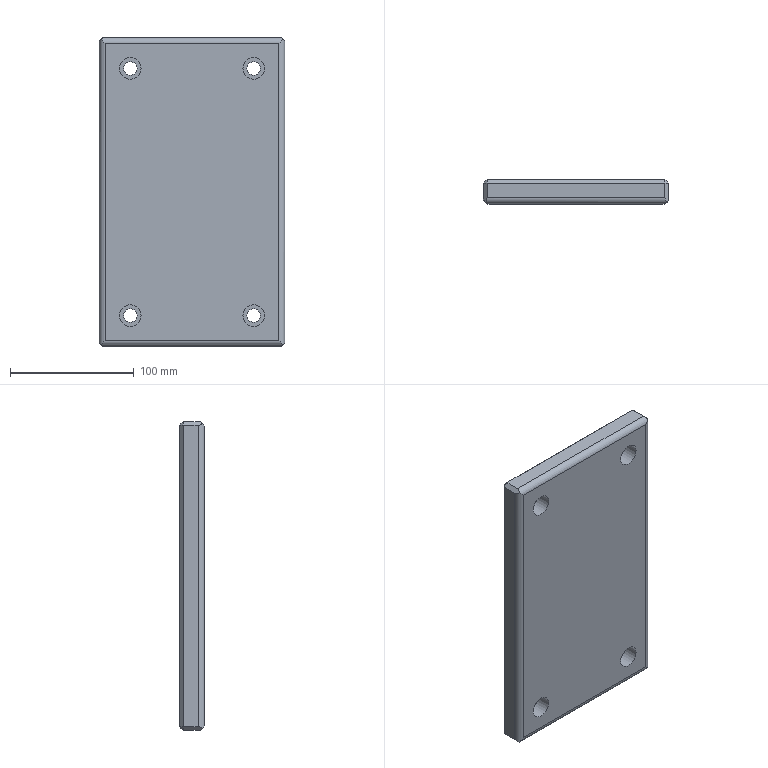Part | NX | features MAIN_BODY 2 | 1 solid | 34 faces | box 150 x 20 x 250 mm | volume 727336 mm3 | plane 22 | cylinder 12 | commonest cylinder face diameters 10 x4 11 x4 17.5 x4
STEP:
#1=CARTESIAN_POINT('',(1390.5,-413.,-220.));
#2=VERTEX_POINT('',#1);
#3=CARTESIAN_POINT('',(1390.5,-425.,-220.));
#4=VERTEX_POINT('',#3);
#5=CARTESIAN_POINT('',(1390.5,-410.,-220.));
#6=DIRECTION('',(0.,-1.,0.));
#7=VECTOR('',#6,1000.);
#8=LINE('',#5,#7);
#9=EDGE_CURVE('',#2,#4,#8,.T.);
#10=ORIENTED_EDGE('',*,*,#9,.F.);
#11=CARTESIAN_POINT('',(1534.5,-413.,-220.));
#12=VERTEX_POINT('',#11);
#13=CARTESIAN_POINT('',(1387.5,-413.,-220.));
#14=DIRECTION('',(-1.,0.,0.));
#15=VECTOR('',#14,1000.);
#16=LINE('',#13,#15);
#17=EDGE_CURVE('',#12,#2,#16,.T.);
#18=ORIENTED_EDGE('',*,*,#17,.F.);
#19=CARTESIAN_POINT('',(1534.5,-425.,-220.));
#20=VERTEX_POINT('',#19);
#21=CARTESIAN_POINT('',(1534.5,-410.,-220.));
#22=DIRECTION('',(0.,1.,0.));
#23=VECTOR('',#22,1000.);
#24=LINE('',#21,#23);
#25=EDGE_CURVE('',#20,#12,#24,.T.);
#26=ORIENTED_EDGE('',*,*,#25,.F.);
#27=CARTESIAN_POINT('',(1534.5,-425.,-220.));
#28=DIRECTION('',(1.,0.,0.));
#29=VECTOR('',#28,1000.);
#30=LINE('',#27,#29);
#31=EDGE_CURVE('',#4,#20,#30,.T.);
#32=ORIENTED_EDGE('',*,*,#31,.F.);
#33=EDGE_LOOP('',(#10,#18,#26,#32));
#34=FACE_BOUND('',#33,.T.);
#35=CARTESIAN_POINT('',(1387.5,-410.,-220.));
#36=DIRECTION('',(0.,0.,1.));
#37=DIRECTION('',(0.,1.,0.));
#38=AXIS2_PLACEMENT_3D('',#35,#36,#37);
#39=PLANE('',#38);
#40=ADVANCED_FACE('',(#34),#39,.F.);
#41=CARTESIAN_POINT('',(1537.5,-413.,-217.));
#42=VERTEX_POINT('',#41);
#43=CARTESIAN_POINT('',(1537.5,-425.,-217.));
#44=VERTEX_POINT('',#43);
#45=CARTESIAN_POINT('',(1537.5,-410.,-217.));
#46=DIRECTION('',(0.,-1.,0.));
#47=VECTOR('',#46,1000.);
#48=LINE('',#45,#47);
#49=EDGE_CURVE('',#42,#44,#48,.T.);
#50=ORIENTED_EDGE('',*,*,#49,.F.);
#51=CARTESIAN_POINT('',(1537.5,-413.,27.));
#52=VERTEX_POINT('',#51);
#53=CARTESIAN_POINT('',(1537.5,-413.,-220.));
#54=DIRECTION('',(0.,0.,-1.));
#55=VECTOR('',#54,1000.);
#56=LINE('',#53,#55);
#57=EDGE_CURVE('',#52,#42,#56,.T.);
#58=ORIENTED_EDGE('',*,*,#57,.F.);
#59=CARTESIAN_POINT('',(1537.5,-425.,27.));
#60=VERTEX_POINT('',#59);
#61=CARTESIAN_POINT('',(1537.5,-410.,27.));
#62=DIRECTION('',(0.,1.,0.));
#63=VECTOR('',#62,1000.);
#64=LINE('',#61,#63);
#65=EDGE_CURVE('',#60,#52,#64,.T.);
#66=ORIENTED_EDGE('',*,*,#65,.F.);
#67=CARTESIAN_POINT('',(1537.5,-425.,27.));
#68=DIRECTION('',(0.,0.,1.));
#69=VECTOR('',#68,1000.);
#70=LINE('',#67,#69);
#71=EDGE_CURVE('',#44,#60,#70,.T.);
#72=ORIENTED_EDGE('',*,*,#71,.F.);
#73=EDGE_LOOP('',(#50,#58,#66,#72));
#74=FACE_BOUND('',#73,.T.);
#75=CARTESIAN_POINT('',(1537.5,-410.,-220.));
#76=DIRECTION('',(-1.,0.,0.));
#77=DIRECTION('',(0.,0.,1.));
#78=AXIS2_PLACEMENT_3D('',#75,#76,#77);
#79=PLANE('',#78);
#80=ADVANCED_FACE('',(#74),#79,.F.);
#81=CARTESIAN_POINT('',(1534.5,-413.,30.));
#82=VERTEX_POINT('',#81);
#83=CARTESIAN_POINT('',(1534.5,-425.,30.));
#84=VERTEX_POINT('',#83);
#85=CARTESIAN_POINT('',(1534.5,-410.,30.));
#86=DIRECTION('',(0.,-1.,0.));
#87=VECTOR('',#86,1000.);
#88=LINE('',#85,#87);
#89=EDGE_CURVE('',#82,#84,#88,.T.);
#90=ORIENTED_EDGE('',*,*,#89,.F.);
#91=CARTESIAN_POINT('',(1390.5,-413.,30.));
#92=VERTEX_POINT('',#91);
#93=CARTESIAN_POINT('',(1537.5,-413.,30.));
#94=DIRECTION('',(1.,0.,0.));
#95=VECTOR('',#94,1000.);
#96=LINE('',#93,#95);
#97=EDGE_CURVE('',#92,#82,#96,.T.);
#98=ORIENTED_EDGE('',*,*,#97,.F.);
#99=CARTESIAN_POINT('',(1390.5,-425.,30.));
#100=VERTEX_POINT('',#99);
#101=CARTESIAN_POINT('',(1390.5,-410.,30.));
#102=DIRECTION('',(0.,1.,0.));
#103=VECTOR('',#102,1000.);
#104=LINE('',#101,#103);
#105=EDGE_CURVE('',#100,#92,#104,.T.);
#106=ORIENTED_EDGE('',*,*,#105,.F.);
#107=CARTESIAN_POINT('',(1390.5,-425.,30.));
#108=DIRECTION('',(-1.,0.,0.));
#109=VECTOR('',#108,1000.);
#110=LINE('',#107,#109);
#111=EDGE_CURVE('',#84,#100,#110,.T.);
#112=ORIENTED_EDGE('',*,*,#111,.F.);
#113=EDGE_LOOP('',(#90,#98,#106,#112));
#114=FACE_BOUND('',#113,.T.);
#115=CARTESIAN_POINT('',(1537.5,-410.,30.));
#116=DIRECTION('',(0.,0.,-1.));
#117=DIRECTION('',(-1.,0.,0.));
#118=AXIS2_PLACEMENT_3D('',#115,#116,#117);
#119=PLANE('',#118);
#120=ADVANCED_FACE('',(#114),#119,.F.);
#121=CARTESIAN_POINT('',(1387.5,-413.,27.));
#122=VERTEX_POINT('',#121);
#123=CARTESIAN_POINT('',(1387.5,-425.,27.));
#124=VERTEX_POINT('',#123);
#125=CARTESIAN_POINT('',(1387.5,-410.,27.));
#126=DIRECTION('',(0.,-1.,0.));
#127=VECTOR('',#126,1000.);
#128=LINE('',#125,#127);
#129=EDGE_CURVE('',#122,#124,#128,.T.);
#130=ORIENTED_EDGE('',*,*,#129,.F.);
#131=CARTESIAN_POINT('',(1387.5,-413.,-217.));
#132=VERTEX_POINT('',#131);
#133=CARTESIAN_POINT('',(1387.5,-413.,30.));
#134=DIRECTION('',(0.,0.,1.));
#135=VECTOR('',#134,1000.);
#136=LINE('',#133,#135);
#137=EDGE_CURVE('',#132,#122,#136,.T.);
#138=ORIENTED_EDGE('',*,*,#137,.F.);
#139=CARTESIAN_POINT('',(1387.5,-425.,-217.));
#140=VERTEX_POINT('',#139);
#141=CARTESIAN_POINT('',(1387.5,-410.,-217.));
#142=DIRECTION('',(0.,1.,0.));
#143=VECTOR('',#142,1000.);
#144=LINE('',#141,#143);
#145=EDGE_CURVE('',#140,#132,#144,.T.);
#146=ORIENTED_EDGE('',*,*,#145,.F.);
#147=CARTESIAN_POINT('',(1387.5,-425.,-217.));
#148=DIRECTION('',(0.,0.,-1.));
#149=VECTOR('',#148,1000.);
#150=LINE('',#147,#149);
#151=EDGE_CURVE('',#124,#140,#150,.T.);
#152=ORIENTED_EDGE('',*,*,#151,.F.);
#153=EDGE_LOOP('',(#130,#138,#146,#152));
#154=FACE_BOUND('',#153,.T.);
#155=CARTESIAN_POINT('',(1387.5,-410.,30.));
#156=DIRECTION('',(1.,0.,0.));
#157=DIRECTION('',(0.,0.,-1.));
#158=AXIS2_PLACEMENT_3D('',#155,#156,#157);
#159=PLANE('',#158);
#160=ADVANCED_FACE('',(#154),#159,.F.);
#161=CARTESIAN_POINT('',(1390.5,-410.,27.));
#162=VERTEX_POINT('',#161);
#163=CARTESIAN_POINT('',(1390.5,-410.,-217.));
#164=VERTEX_POINT('',#163);
#165=CARTESIAN_POINT('',(1390.5,-410.,-220.));
#166=DIRECTION('',(0.,0.,-1.));
#167=VECTOR('',#166,1000.);
#168=LINE('',#165,#167);
#169=EDGE_CURVE('',#162,#164,#168,.T.);
#170=ORIENTED_EDGE('',*,*,#169,.F.);
#171=CARTESIAN_POINT('',(1534.5,-410.,27.));
#172=VERTEX_POINT('',#171);
#173=CARTESIAN_POINT('',(1387.5,-410.,27.));
#174=DIRECTION('',(-1.,0.,0.));
#175=VECTOR('',#174,1000.);
#176=LINE('',#173,#175);
#177=EDGE_CURVE('',#172,#162,#176,.T.);
#178=ORIENTED_EDGE('',*,*,#177,.F.);
#179=CARTESIAN_POINT('',(1534.5,-410.,-217.));
#180=VERTEX_POINT('',#179);
#181=CARTESIAN_POINT('',(1534.5,-410.,-220.));
#182=DIRECTION('',(0.,0.,1.));
#183=VECTOR('',#182,1000.);
#184=LINE('',#181,#183);
#185=EDGE_CURVE('',#180,#172,#184,.T.);
#186=ORIENTED_EDGE('',*,*,#185,.F.);
#187=CARTESIAN_POINT('',(1387.5,-410.,-217.));
#188=DIRECTION('',(1.,0.,0.));
#189=VECTOR('',#188,1000.);
#190=LINE('',#187,#189);
#191=EDGE_CURVE('',#164,#180,#190,.T.);
#192=ORIENTED_EDGE('',*,*,#191,.F.);
#193=EDGE_LOOP('',(#170,#178,#186,#192));
#194=FACE_BOUND('',#193,.T.);
#195=CARTESIAN_POINT('',(1518.,-410.,-195.));
#196=VERTEX_POINT('',#195);
#197=CARTESIAN_POINT('',(1512.5,-410.,-195.));
#198=DIRECTION('',(0.,1.,0.));
#199=DIRECTION('',(1.,0.,0.));
#200=AXIS2_PLACEMENT_3D('',#197,#198,#199);
#201=CIRCLE('',#200,5.5);
#202=EDGE_CURVE('',#196,#196,#201,.T.);
#203=ORIENTED_EDGE('',*,*,#202,.F.);
#204=EDGE_LOOP('',(#203));
#205=FACE_BOUND('',#204,.T.);
#206=CARTESIAN_POINT('',(1418.,-410.,-195.));
#207=VERTEX_POINT('',#206);
#208=CARTESIAN_POINT('',(1412.5,-410.,-195.));
#209=DIRECTION('',(0.,1.,0.));
#210=DIRECTION('',(1.,0.,0.));
#211=AXIS2_PLACEMENT_3D('',#208,#209,#210);
#212=CIRCLE('',#211,5.5);
#213=EDGE_CURVE('',#207,#207,#212,.T.);
#214=ORIENTED_EDGE('',*,*,#213,.F.);
#215=EDGE_LOOP('',(#214));
#216=FACE_BOUND('',#215,.T.);
#217=CARTESIAN_POINT('',(1418.,-410.,5.));
#218=VERTEX_POINT('',#217);
#219=CARTESIAN_POINT('',(1412.5,-410.,5.));
#220=DIRECTION('',(0.,1.,0.));
#221=DIRECTION('',(1.,0.,0.));
#222=AXIS2_PLACEMENT_3D('',#219,#220,#221);
#223=CIRCLE('',#222,5.5);
#224=EDGE_CURVE('',#218,#218,#223,.T.);
#225=ORIENTED_EDGE('',*,*,#224,.F.);
#226=EDGE_LOOP('',(#225));
#227=FACE_BOUND('',#226,.T.);
#228=CARTESIAN_POINT('',(1518.,-410.,5.));
#229=VERTEX_POINT('',#228);
#230=CARTESIAN_POINT('',(1512.5,-410.,5.));
#231=DIRECTION('',(0.,1.,0.));
#232=DIRECTION('',(1.,0.,0.));
#233=AXIS2_PLACEMENT_3D('',#230,#231,#232);
#234=CIRCLE('',#233,5.5);
#235=EDGE_CURVE('',#229,#229,#234,.T.);
#236=ORIENTED_EDGE('',*,*,#235,.F.);
#237=EDGE_LOOP('',(#236));
#238=FACE_BOUND('',#237,.T.);
#239=CARTESIAN_POINT('',(1387.5,-410.,-220.));
#240=DIRECTION('',(0.,-1.,0.));
#241=DIRECTION('',(1.,0.,0.));
#242=AXIS2_PLACEMENT_3D('',#239,#240,#241);
#243=PLANE('',#242);
#244=ADVANCED_FACE('',(#194,#205,#216,#227,#238),#243,.F.);
#245=CARTESIAN_POINT('',(1392.5,-430.,25.));
#246=VERTEX_POINT('',#245);
#247=CARTESIAN_POINT('',(1532.5,-430.,25.));
#248=VERTEX_POINT('',#247);
#249=CARTESIAN_POINT('',(1534.5,-430.,25.));
#250=DIRECTION('',(-1.,0.,0.));
#251=VECTOR('',#250,1000.);
#252=LINE('',#249,#251);
#253=EDGE_CURVE('',#246,#248,#252,.F.);
#254=ORIENTED_EDGE('',*,*,#253,.F.);
#255=CARTESIAN_POINT('',(1392.5,-430.,-215.));
#256=VERTEX_POINT('',#255);
#257=CARTESIAN_POINT('',(1392.5,-430.,27.));
#258=DIRECTION('',(0.,0.,-1.));
#259=VECTOR('',#258,1000.);
#260=LINE('',#257,#259);
#261=EDGE_CURVE('',#256,#246,#260,.F.);
#262=ORIENTED_EDGE('',*,*,#261,.F.);
#263=CARTESIAN_POINT('',(1532.5,-430.,-215.));
#264=VERTEX_POINT('',#263);
#265=CARTESIAN_POINT('',(1390.5,-430.,-215.));
#266=DIRECTION('',(1.,0.,0.));
#267=VECTOR('',#266,1000.);
#268=LINE('',#265,#267);
#269=EDGE_CURVE('',#264,#256,#268,.F.);
#270=ORIENTED_EDGE('',*,*,#269,.F.);
#271=CARTESIAN_POINT('',(1532.5,-430.,-217.));
#272=DIRECTION('',(0.,0.,1.));
#273=VECTOR('',#272,1000.);
#274=LINE('',#271,#273);
#275=EDGE_CURVE('',#248,#264,#274,.F.);
#276=ORIENTED_EDGE('',*,*,#275,.F.);
#277=EDGE_LOOP('',(#254,#262,#270,#276));
#278=FACE_BOUND('',#277,.T.);
#279=CARTESIAN_POINT('',(1503.75,-430.,-195.));
#280=VERTEX_POINT('',#279);
#281=CARTESIAN_POINT('',(1512.5,-430.,-195.));
#282=DIRECTION('',(0.,-1.,0.));
#283=DIRECTION('',(-1.,0.,0.));
#284=AXIS2_PLACEMENT_3D('',#281,#282,#283);
#285=CIRCLE('',#284,8.75);
#286=EDGE_CURVE('',#280,#280,#285,.T.);
#287=ORIENTED_EDGE('',*,*,#286,.F.);
#288=EDGE_LOOP('',(#287));
#289=FACE_BOUND('',#288,.T.);
#290=CARTESIAN_POINT('',(1403.75,-430.,-195.));
#291=VERTEX_POINT('',#290);
#292=CARTESIAN_POINT('',(1412.5,-430.,-195.));
#293=DIRECTION('',(0.,-1.,0.));
#294=DIRECTION('',(-1.,0.,0.));
#295=AXIS2_PLACEMENT_3D('',#292,#293,#294);
#296=CIRCLE('',#295,8.75);
#297=EDGE_CURVE('',#291,#291,#296,.T.);
#298=ORIENTED_EDGE('',*,*,#297,.F.);
#299=EDGE_LOOP('',(#298));
#300=FACE_BOUND('',#299,.T.);
#301=CARTESIAN_POINT('',(1403.75,-430.,5.));
#302=VERTEX_POINT('',#301);
#303=CARTESIAN_POINT('',(1412.5,-430.,5.));
#304=DIRECTION('',(0.,-1.,0.));
#305=DIRECTION('',(-1.,0.,0.));
#306=AXIS2_PLACEMENT_3D('',#303,#304,#305);
#307=CIRCLE('',#306,8.75);
#308=EDGE_CURVE('',#302,#302,#307,.T.);
#309=ORIENTED_EDGE('',*,*,#308,.F.);
#310=EDGE_LOOP('',(#309));
#311=FACE_BOUND('',#310,.T.);
#312=CARTESIAN_POINT('',(1503.75,-430.,5.));
#313=VERTEX_POINT('',#312);
#314=CARTESIAN_POINT('',(1512.5,-430.,5.));
#315=DIRECTION('',(0.,-1.,0.));
#316=DIRECTION('',(-1.,0.,0.));
#317=AXIS2_PLACEMENT_3D('',#314,#315,#316);
#318=CIRCLE('',#317,8.75);
#319=EDGE_CURVE('',#313,#313,#318,.T.);
#320=ORIENTED_EDGE('',*,*,#319,.F.);
#321=EDGE_LOOP('',(#320));
#322=FACE_BOUND('',#321,.T.);
#323=CARTESIAN_POINT('',(1387.5,-430.,-220.));
#324=DIRECTION('',(0.,-1.,0.));
#325=DIRECTION('',(1.,0.,0.));
#326=AXIS2_PLACEMENT_3D('',#323,#324,#325);
#327=PLANE('',#326);
#328=ADVANCED_FACE('',(#278,#289,#300,#311,#322),#327,.T.);
#329=CARTESIAN_POINT('',(1507.,-418.,5.));
#330=VERTEX_POINT('',#329);
#331=CARTESIAN_POINT('',(1512.5,-418.,5.));
#332=DIRECTION('',(0.,-1.,0.));
#333=DIRECTION('',(-1.,0.,0.));
#334=AXIS2_PLACEMENT_3D('',#331,#332,#333);
#335=CIRCLE('',#334,5.5);
#336=EDGE_CURVE('',#330,#330,#335,.T.);
#337=ORIENTED_EDGE('',*,*,#336,.T.);
#338=EDGE_LOOP('',(#337));
#339=FACE_BOUND('',#338,.T.);
#340=ORIENTED_EDGE('',*,*,#235,.T.);
#341=EDGE_LOOP('',(#340));
#342=FACE_BOUND('',#341,.T.);
#343=CARTESIAN_POINT('',(1512.5,-380.,5.));
#344=DIRECTION('',(0.,1.,0.));
#345=DIRECTION('',(-1.,0.,0.));
#346=AXIS2_PLACEMENT_3D('',#343,#344,#345);
#347=CYLINDRICAL_SURFACE('',#346,5.5);
#348=ADVANCED_FACE('',(#339,#342),#347,.F.);
#349=ORIENTED_EDGE('',*,*,#336,.F.);
#350=EDGE_LOOP('',(#349));
#351=FACE_BOUND('',#350,.T.);
#352=CARTESIAN_POINT('',(1503.75,-418.,5.));
#353=VERTEX_POINT('',#352);
#354=CARTESIAN_POINT('',(1512.5,-418.,5.));
#355=DIRECTION('',(0.,-1.,0.));
#356=DIRECTION('',(-1.,0.,0.));
#357=AXIS2_PLACEMENT_3D('',#354,#355,#356);
#358=CIRCLE('',#357,8.75);
#359=EDGE_CURVE('',#353,#353,#358,.T.);
#360=ORIENTED_EDGE('',*,*,#359,.T.);
#361=EDGE_LOOP('',(#360));
#362=FACE_BOUND('',#361,.T.);
#363=CARTESIAN_POINT('',(1512.5,-418.,5.));
#364=DIRECTION('',(0.,1.,0.));
#365=DIRECTION('',(-1.,0.,0.));
#366=AXIS2_PLACEMENT_3D('',#363,#364,#365);
#367=PLANE('',#366);
#368=ADVANCED_FACE('',(#351,#362),#367,.F.);
#369=ORIENTED_EDGE('',*,*,#359,.F.);
#370=EDGE_LOOP('',(#369));
#371=FACE_BOUND('',#370,.T.);
#372=ORIENTED_EDGE('',*,*,#319,.T.);
#373=EDGE_LOOP('',(#372));
#374=FACE_BOUND('',#373,.T.);
#375=CARTESIAN_POINT('',(1512.5,-430.,5.));
#376=DIRECTION('',(0.,1.,0.));
#377=DIRECTION('',(-1.,0.,0.));
#378=AXIS2_PLACEMENT_3D('',#375,#376,#377);
#379=CYLINDRICAL_SURFACE('',#378,8.75);
#380=ADVANCED_FACE('',(#371,#374),#379,.F.);
#381=CARTESIAN_POINT('',(1407.,-418.,5.));
#382=VERTEX_POINT('',#381);
#383=CARTESIAN_POINT('',(1412.5,-418.,5.));
#384=DIRECTION('',(0.,-1.,0.));
#385=DIRECTION('',(-1.,0.,0.));
#386=AXIS2_PLACEMENT_3D('',#383,#384,#385);
#387=CIRCLE('',#386,5.5);
#388=EDGE_CURVE('',#382,#382,#387,.T.);
#389=ORIENTED_EDGE('',*,*,#388,.T.);
#390=EDGE_LOOP('',(#389));
#391=FACE_BOUND('',#390,.T.);
#392=ORIENTED_EDGE('',*,*,#224,.T.);
#393=EDGE_LOOP('',(#392));
#394=FACE_BOUND('',#393,.T.);
#395=CARTESIAN_POINT('',(1412.5,-380.,5.));
#396=DIRECTION('',(0.,1.,0.));
#397=DIRECTION('',(-1.,0.,0.));
#398=AXIS2_PLACEMENT_3D('',#395,#396,#397);
#399=CYLINDRICAL_SURFACE('',#398,5.5);
#400=ADVANCED_FACE('',(#391,#394),#399,.F.);
#401=ORIENTED_EDGE('',*,*,#388,.F.);
#402=EDGE_LOOP('',(#401));
#403=FACE_BOUND('',#402,.T.);
#404=CARTESIAN_POINT('',(1403.75,-418.,5.));
#405=VERTEX_POINT('',#404);
#406=CARTESIAN_POINT('',(1412.5,-418.,5.));
#407=DIRECTION('',(0.,-1.,0.));
#408=DIRECTION('',(-1.,0.,0.));
#409=AXIS2_PLACEMENT_3D('',#406,#407,#408);
#410=CIRCLE('',#409,8.75);
#411=EDGE_CURVE('',#405,#405,#410,.T.);
#412=ORIENTED_EDGE('',*,*,#411,.T.);
#413=EDGE_LOOP('',(#412));
#414=FACE_BOUND('',#413,.T.);
#415=CARTESIAN_POINT('',(1412.5,-418.,5.));
#416=DIRECTION('',(0.,1.,0.));
#417=DIRECTION('',(-1.,0.,0.));
#418=AXIS2_PLACEMENT_3D('',#415,#416,#417);
#419=PLANE('',#418);
#420=ADVANCED_FACE('',(#403,#414),#419,.F.);
#421=ORIENTED_EDGE('',*,*,#411,.F.);
#422=EDGE_LOOP('',(#421));
#423=FACE_BOUND('',#422,.T.);
#424=ORIENTED_EDGE('',*,*,#308,.T.);
#425=EDGE_LOOP('',(#424));
#426=FACE_BOUND('',#425,.T.);
#427=CARTESIAN_POINT('',(1412.5,-430.,5.));
#428=DIRECTION('',(0.,1.,0.));
#429=DIRECTION('',(-1.,0.,0.));
#430=AXIS2_PLACEMENT_3D('',#427,#428,#429);
#431=CYLINDRICAL_SURFACE('',#430,8.75);
#432=ADVANCED_FACE('',(#423,#426),#431,.F.);
#433=CARTESIAN_POINT('',(1407.,-418.,-195.));
#434=VERTEX_POINT('',#433);
#435=CARTESIAN_POINT('',(1412.5,-418.,-195.));
#436=DIRECTION('',(0.,-1.,0.));
#437=DIRECTION('',(-1.,0.,0.));
#438=AXIS2_PLACEMENT_3D('',#435,#436,#437);
#439=CIRCLE('',#438,5.5);
#440=EDGE_CURVE('',#434,#434,#439,.T.);
#441=ORIENTED_EDGE('',*,*,#440,.T.);
#442=EDGE_LOOP('',(#441));
#443=FACE_BOUND('',#442,.T.);
#444=ORIENTED_EDGE('',*,*,#213,.T.);
#445=EDGE_LOOP('',(#444));
#446=FACE_BOUND('',#445,.T.);
#447=CARTESIAN_POINT('',(1412.5,-380.,-195.));
#448=DIRECTION('',(0.,1.,0.));
#449=DIRECTION('',(-1.,0.,0.));
#450=AXIS2_PLACEMENT_3D('',#447,#448,#449);
#451=CYLINDRICAL_SURFACE('',#450,5.5);
#452=ADVANCED_FACE('',(#443,#446),#451,.F.);
#453=ORIENTED_EDGE('',*,*,#440,.F.);
#454=EDGE_LOOP('',(#453));
#455=FACE_BOUND('',#454,.T.);
#456=CARTESIAN_POINT('',(1403.75,-418.,-195.));
#457=VERTEX_POINT('',#456);
#458=CARTESIAN_POINT('',(1412.5,-418.,-195.));
#459=DIRECTION('',(0.,-1.,0.));
#460=DIRECTION('',(-1.,0.,0.));
#461=AXIS2_PLACEMENT_3D('',#458,#459,#460);
#462=CIRCLE('',#461,8.75);
#463=EDGE_CURVE('',#457,#457,#462,.T.);
#464=ORIENTED_EDGE('',*,*,#463,.T.);
#465=EDGE_LOOP('',(#464));
#466=FACE_BOUND('',#465,.T.);
#467=CARTESIAN_POINT('',(1412.5,-418.,-195.));
#468=DIRECTION('',(0.,1.,0.));
#469=DIRECTION('',(-1.,0.,0.));
#470=AXIS2_PLACEMENT_3D('',#467,#468,#469);
#471=PLANE('',#470);
#472=ADVANCED_FACE('',(#455,#466),#471,.F.);
#473=ORIENTED_EDGE('',*,*,#463,.F.);
#474=EDGE_LOOP('',(#473));
#475=FACE_BOUND('',#474,.T.);
#476=ORIENTED_EDGE('',*,*,#297,.T.);
#477=EDGE_LOOP('',(#476));
#478=FACE_BOUND('',#477,.T.);
#479=CARTESIAN_POINT('',(1412.5,-430.,-195.));
#480=DIRECTION('',(0.,1.,0.));
#481=DIRECTION('',(-1.,0.,0.));
#482=AXIS2_PLACEMENT_3D('',#479,#480,#481);
#483=CYLINDRICAL_SURFACE('',#482,8.75);
#484=ADVANCED_FACE('',(#475,#478),#483,.F.);
#485=CARTESIAN_POINT('',(1507.,-418.,-195.));
#486=VERTEX_POINT('',#485);
#487=CARTESIAN_POINT('',(1512.5,-418.,-195.));
#488=DIRECTION('',(0.,-1.,0.));
#489=DIRECTION('',(-1.,0.,0.));
#490=AXIS2_PLACEMENT_3D('',#487,#488,#489);
#491=CIRCLE('',#490,5.5);
#492=EDGE_CURVE('',#486,#486,#491,.T.);
#493=ORIENTED_EDGE('',*,*,#492,.T.);
#494=EDGE_LOOP('',(#493));
#495=FACE_BOUND('',#494,.T.);
#496=ORIENTED_EDGE('',*,*,#202,.T.);
#497=EDGE_LOOP('',(#496));
#498=FACE_BOUND('',#497,.T.);
#499=CARTESIAN_POINT('',(1512.5,-380.,-195.));
#500=DIRECTION('',(0.,1.,0.));
#501=DIRECTION('',(-1.,0.,0.));
#502=AXIS2_PLACEMENT_3D('',#499,#500,#501);
#503=CYLINDRICAL_SURFACE('',#502,5.5);
#504=ADVANCED_FACE('',(#495,#498),#503,.F.);
#505=ORIENTED_EDGE('',*,*,#492,.F.);
#506=EDGE_LOOP('',(#505));
#507=FACE_BOUND('',#506,.T.);
#508=CARTESIAN_POINT('',(1503.75,-418.,-195.));
#509=VERTEX_POINT('',#508);
#510=CARTESIAN_POINT('',(1512.5,-418.,-195.));
#511=DIRECTION('',(0.,-1.,0.));
#512=DIRECTION('',(-1.,0.,0.));
#513=AXIS2_PLACEMENT_3D('',#510,#511,#512);
#514=CIRCLE('',#513,8.75);
#515=EDGE_CURVE('',#509,#509,#514,.T.);
#516=ORIENTED_EDGE('',*,*,#515,.T.);
#517=EDGE_LOOP('',(#516));
#518=FACE_BOUND('',#517,.T.);
#519=CARTESIAN_POINT('',(1512.5,-418.,-195.));
#520=DIRECTION('',(0.,1.,0.));
#521=DIRECTION('',(-1.,0.,0.));
#522=AXIS2_PLACEMENT_3D('',#519,#520,#521);
#523=PLANE('',#522);
#524=ADVANCED_FACE('',(#507,#518),#523,.F.);
#525=ORIENTED_EDGE('',*,*,#515,.F.);
#526=EDGE_LOOP('',(#525));
#527=FACE_BOUND('',#526,.T.);
#528=ORIENTED_EDGE('',*,*,#286,.T.);
#529=EDGE_LOOP('',(#528));
#530=FACE_BOUND('',#529,.T.);
#531=CARTESIAN_POINT('',(1512.5,-430.,-195.));
#532=DIRECTION('',(0.,1.,0.));
#533=DIRECTION('',(-1.,0.,0.));
#534=AXIS2_PLACEMENT_3D('',#531,#532,#533);
#535=CYLINDRICAL_SURFACE('',#534,8.75);
#536=ADVANCED_FACE('',(#527,#530),#535,.F.);
#537=CARTESIAN_POINT('',(1389.,-428.571,28.5));
#538=VERTEX_POINT('',#537);
#539=CARTESIAN_POINT('',(1385.5,-425.,25.));
#540=DIRECTION('',(-0.7071,0.,0.7071));
#541=DIRECTION('',(0.7071,0.,0.7071));
#542=AXIS2_PLACEMENT_3D('',#539,#540,#541);
#543=ELLIPSE('',#542,7.071,5.);
#544=EDGE_CURVE('',#100,#538,#543,.F.);
#545=ORIENTED_EDGE('',*,*,#544,.F.);
#546=ORIENTED_EDGE('',*,*,#105,.T.);
#547=CARTESIAN_POINT('',(1387.5,-413.,27.));
#548=DIRECTION('',(0.7071,0.,0.7071));
#549=VECTOR('',#548,1000.);
#550=LINE('',#547,#549);
#551=EDGE_CURVE('',#92,#122,#550,.F.);
#552=ORIENTED_EDGE('',*,*,#551,.T.);
#553=ORIENTED_EDGE('',*,*,#129,.T.);
#554=CARTESIAN_POINT('',(1392.5,-425.,32.));
#555=DIRECTION('',(-0.7071,0.,0.7071));
#556=DIRECTION('',(0.7071,0.,0.7071));
#557=AXIS2_PLACEMENT_3D('',#554,#555,#556);
#558=ELLIPSE('',#557,7.071,5.);
#559=EDGE_CURVE('',#538,#124,#558,.F.);
#560=ORIENTED_EDGE('',*,*,#559,.F.);
#561=EDGE_LOOP('',(#545,#546,#552,#553,#560));
#562=FACE_BOUND('',#561,.T.);
#563=CARTESIAN_POINT('',(1387.5,-410.,27.));
#564=DIRECTION('',(0.7071,0.,-0.7071));
#565=DIRECTION('',(-0.7071,0.,-0.7071));
#566=AXIS2_PLACEMENT_3D('',#563,#564,#565);
#567=PLANE('',#566);
#568=ADVANCED_FACE('',(#562),#567,.F.);
#569=CARTESIAN_POINT('',(1534.5,-413.,30.));
#570=DIRECTION('',(0.,-0.7071,0.7071));
#571=VECTOR('',#570,1000.);
#572=LINE('',#569,#571);
#573=EDGE_CURVE('',#82,#172,#572,.F.);
#574=ORIENTED_EDGE('',*,*,#573,.T.);
#575=ORIENTED_EDGE('',*,*,#177,.T.);
#576=CARTESIAN_POINT('',(1390.5,-411.5,28.5));
#577=DIRECTION('',(0.,0.7071,-0.7071));
#578=VECTOR('',#577,1000.);
#579=LINE('',#576,#578);
#580=EDGE_CURVE('',#162,#92,#579,.F.);
#581=ORIENTED_EDGE('',*,*,#580,.T.);
#582=ORIENTED_EDGE('',*,*,#97,.T.);
#583=EDGE_LOOP('',(#574,#575,#581,#582));
#584=FACE_BOUND('',#583,.T.);
#585=CARTESIAN_POINT('',(1387.5,-410.,27.));
#586=DIRECTION('',(0.,-0.7071,-0.7071));
#587=DIRECTION('',(0.,-0.7071,0.7071));
#588=AXIS2_PLACEMENT_3D('',#585,#586,#587);
#589=PLANE('',#588);
#590=ADVANCED_FACE('',(#584),#589,.F.);
#591=ORIENTED_EDGE('',*,*,#65,.T.);
#592=CARTESIAN_POINT('',(1534.5,-413.,30.));
#593=DIRECTION('',(0.7071,0.,-0.7071));
#594=VECTOR('',#593,1000.);
#595=LINE('',#592,#594);
#596=EDGE_CURVE('',#52,#82,#595,.F.);
#597=ORIENTED_EDGE('',*,*,#596,.T.);
#598=ORIENTED_EDGE('',*,*,#89,.T.);
#599=CARTESIAN_POINT('',(1536.,-428.571,28.5));
#600=VERTEX_POINT('',#599);
#601=CARTESIAN_POINT('',(1539.5,-425.,25.));
#602=DIRECTION('',(0.7071,0.,0.7071));
#603=DIRECTION('',(0.7071,0.,-0.7071));
#604=AXIS2_PLACEMENT_3D('',#601,#602,#603);
#605=ELLIPSE('',#604,7.071,5.);
#606=EDGE_CURVE('',#600,#84,#605,.F.);
#607=ORIENTED_EDGE('',*,*,#606,.F.);
#608=CARTESIAN_POINT('',(1532.5,-425.,32.));
#609=DIRECTION('',(0.7071,0.,0.7071));
#610=DIRECTION('',(0.7071,0.,-0.7071));
#611=AXIS2_PLACEMENT_3D('',#608,#609,#610);
#612=ELLIPSE('',#611,7.071,5.);
#613=EDGE_CURVE('',#60,#600,#612,.F.);
#614=ORIENTED_EDGE('',*,*,#613,.F.);
#615=EDGE_LOOP('',(#591,#597,#598,#607,#614));
#616=FACE_BOUND('',#615,.T.);
#617=CARTESIAN_POINT('',(1534.5,-410.,30.));
#618=DIRECTION('',(-0.7071,0.,-0.7071));
#619=DIRECTION('',(-0.7071,0.,0.7071));
#620=AXIS2_PLACEMENT_3D('',#617,#618,#619);
#621=PLANE('',#620);
#622=ADVANCED_FACE('',(#616),#621,.F.);
#623=ORIENTED_EDGE('',*,*,#580,.F.);
#624=CARTESIAN_POINT('',(1387.5,-413.,27.));
#625=DIRECTION('',(-0.7071,-0.7071,0.));
#626=VECTOR('',#625,1000.);
#627=LINE('',#624,#626);
#628=EDGE_CURVE('',#162,#122,#627,.T.);
#629=ORIENTED_EDGE('',*,*,#628,.T.);
#630=ORIENTED_EDGE('',*,*,#551,.F.);
#631=EDGE_LOOP('',(#623,#629,#630));
#632=FACE_BOUND('',#631,.T.);
#633=CARTESIAN_POINT('',(1387.5,-413.,27.));
#634=DIRECTION('',(-0.5774,0.5774,0.5774));
#635=DIRECTION('',(0.,0.7071,-0.7071));
#636=AXIS2_PLACEMENT_3D('',#633,#634,#635);
#637=PLANE('',#636);
#638=ADVANCED_FACE('',(#632),#637,.T.);
#639=ORIENTED_EDGE('',*,*,#596,.F.);
#640=CARTESIAN_POINT('',(1536.,-411.5,27.));
#641=DIRECTION('',(-0.7071,0.7071,0.));
#642=VECTOR('',#641,1000.);
#643=LINE('',#640,#642);
#644=EDGE_CURVE('',#52,#172,#643,.T.);
#645=ORIENTED_EDGE('',*,*,#644,.T.);
#646=ORIENTED_EDGE('',*,*,#573,.F.);
#647=EDGE_LOOP('',(#639,#645,#646));
#648=FACE_BOUND('',#647,.T.);
#649=CARTESIAN_POINT('',(1534.5,-413.,30.));
#650=DIRECTION('',(0.5774,0.5774,0.5774));
#651=DIRECTION('',(-0.7071,0.7071,0.));
#652=AXIS2_PLACEMENT_3D('',#649,#650,#651);
#653=PLANE('',#652);
#654=ADVANCED_FACE('',(#648),#653,.T.);
#655=CARTESIAN_POINT('',(1389.,-428.571,-218.5));
#656=VERTEX_POINT('',#655);
#657=CARTESIAN_POINT('',(1392.5,-425.,-222.));
#658=DIRECTION('',(-0.7071,0.,-0.7071));
#659=DIRECTION('',(-0.7071,0.,0.7071));
#660=AXIS2_PLACEMENT_3D('',#657,#658,#659);
#661=ELLIPSE('',#660,7.071,5.);
#662=EDGE_CURVE('',#140,#656,#661,.F.);
#663=ORIENTED_EDGE('',*,*,#662,.F.);
#664=ORIENTED_EDGE('',*,*,#145,.T.);
#665=CARTESIAN_POINT('',(1390.5,-413.,-220.));
#666=DIRECTION('',(-0.7071,0.,0.7071));
#667=VECTOR('',#666,1000.);
#668=LINE('',#665,#667);
#669=EDGE_CURVE('',#132,#2,#668,.F.);
#670=ORIENTED_EDGE('',*,*,#669,.T.);
#671=ORIENTED_EDGE('',*,*,#9,.T.);
#672=CARTESIAN_POINT('',(1385.5,-425.,-215.));
#673=DIRECTION('',(-0.7071,0.,-0.7071));
#674=DIRECTION('',(-0.7071,0.,0.7071));
#675=AXIS2_PLACEMENT_3D('',#672,#673,#674);
#676=ELLIPSE('',#675,7.071,5.);
#677=EDGE_CURVE('',#656,#4,#676,.F.);
#678=ORIENTED_EDGE('',*,*,#677,.F.);
#679=EDGE_LOOP('',(#663,#664,#670,#671,#678));
#680=FACE_BOUND('',#679,.T.);
#681=CARTESIAN_POINT('',(1390.5,-410.,-220.));
#682=DIRECTION('',(0.7071,0.,0.7071));
#683=DIRECTION('',(0.7071,0.,-0.7071));
#684=AXIS2_PLACEMENT_3D('',#681,#682,#683);
#685=PLANE('',#684);
#686=ADVANCED_FACE('',(#680),#685,.F.);
#687=ORIENTED_EDGE('',*,*,#628,.F.);
#688=ORIENTED_EDGE('',*,*,#169,.T.);
#689=CARTESIAN_POINT('',(1389.,-411.5,-217.));
#690=DIRECTION('',(0.7071,0.7071,0.));
#691=VECTOR('',#690,1000.);
#692=LINE('',#689,#691);
#693=EDGE_CURVE('',#164,#132,#692,.F.);
#694=ORIENTED_EDGE('',*,*,#693,.T.);
#695=ORIENTED_EDGE('',*,*,#137,.T.);
#696=EDGE_LOOP('',(#687,#688,#694,#695));
#697=FACE_BOUND('',#696,.T.);
#698=CARTESIAN_POINT('',(1390.5,-410.,-220.));
#699=DIRECTION('',(0.7071,-0.7071,0.));
#700=DIRECTION('',(0.7071,0.7071,0.));
#701=AXIS2_PLACEMENT_3D('',#698,#699,#700);
#702=PLANE('',#701);
#703=ADVANCED_FACE('',(#697),#702,.F.);
#704=ORIENTED_EDGE('',*,*,#644,.F.);
#705=ORIENTED_EDGE('',*,*,#57,.T.);
#706=CARTESIAN_POINT('',(1534.5,-410.,-217.));
#707=DIRECTION('',(0.7071,-0.7071,0.));
#708=VECTOR('',#707,1000.);
#709=LINE('',#706,#708);
#710=EDGE_CURVE('',#42,#180,#709,.F.);
#711=ORIENTED_EDGE('',*,*,#710,.T.);
#712=ORIENTED_EDGE('',*,*,#185,.T.);
#713=EDGE_LOOP('',(#704,#705,#711,#712));
#714=FACE_BOUND('',#713,.T.);
#715=CARTESIAN_POINT('',(1534.5,-410.,-220.));
#716=DIRECTION('',(-0.7071,-0.7071,0.));
#717=DIRECTION('',(0.7071,-0.7071,0.));
#718=AXIS2_PLACEMENT_3D('',#715,#716,#717);
#719=PLANE('',#718);
#720=ADVANCED_FACE('',(#714),#719,.F.);
#721=CARTESIAN_POINT('',(1536.,-428.571,-218.5));
#722=VERTEX_POINT('',#721);
#723=CARTESIAN_POINT('',(1539.5,-425.,-215.));
#724=DIRECTION('',(0.7071,0.,-0.7071));
#725=DIRECTION('',(-0.7071,0.,-0.7071));
#726=AXIS2_PLACEMENT_3D('',#723,#724,#725);
#727=ELLIPSE('',#726,7.071,5.);
#728=EDGE_CURVE('',#20,#722,#727,.F.);
#729=ORIENTED_EDGE('',*,*,#728,.F.);
#730=ORIENTED_EDGE('',*,*,#25,.T.);
#731=CARTESIAN_POINT('',(1536.,-413.,-218.5));
#732=DIRECTION('',(-0.7071,0.,-0.7071));
#733=VECTOR('',#732,1000.);
#734=LINE('',#731,#733);
#735=EDGE_CURVE('',#12,#42,#734,.F.);
#736=ORIENTED_EDGE('',*,*,#735,.T.);
#737=ORIENTED_EDGE('',*,*,#49,.T.);
#738=CARTESIAN_POINT('',(1532.5,-425.,-222.));
#739=DIRECTION('',(0.7071,0.,-0.7071));
#740=DIRECTION('',(-0.7071,0.,-0.7071));
#741=AXIS2_PLACEMENT_3D('',#738,#739,#740);
#742=ELLIPSE('',#741,7.071,5.);
#743=EDGE_CURVE('',#722,#44,#742,.F.);
#744=ORIENTED_EDGE('',*,*,#743,.F.);
#745=EDGE_LOOP('',(#729,#730,#736,#737,#744));
#746=FACE_BOUND('',#745,.T.);
#747=CARTESIAN_POINT('',(1537.5,-410.,-217.));
#748=DIRECTION('',(-0.7071,0.,0.7071));
#749=DIRECTION('',(0.7071,0.,0.7071));
#750=AXIS2_PLACEMENT_3D('',#747,#748,#749);
#751=PLANE('',#750);
#752=ADVANCED_FACE('',(#746),#751,.F.);
#753=ORIENTED_EDGE('',*,*,#693,.F.);
#754=CARTESIAN_POINT('',(1390.5,-413.,-220.));
#755=DIRECTION('',(0.,-0.7071,-0.7071));
#756=VECTOR('',#755,1000.);
#757=LINE('',#754,#756);
#758=EDGE_CURVE('',#164,#2,#757,.T.);
#759=ORIENTED_EDGE('',*,*,#758,.T.);
#760=ORIENTED_EDGE('',*,*,#669,.F.);
#761=EDGE_LOOP('',(#753,#759,#760));
#762=FACE_BOUND('',#761,.T.);
#763=CARTESIAN_POINT('',(1390.5,-413.,-220.));
#764=DIRECTION('',(-0.5774,0.5774,-0.5774));
#765=DIRECTION('',(-0.7071,-0.7071,0.));
#766=AXIS2_PLACEMENT_3D('',#763,#764,#765);
#767=PLANE('',#766);
#768=ADVANCED_FACE('',(#762),#767,.T.);
#769=ORIENTED_EDGE('',*,*,#735,.F.);
#770=CARTESIAN_POINT('',(1534.5,-410.,-217.));
#771=DIRECTION('',(0.,0.7071,0.7071));
#772=VECTOR('',#771,1000.);
#773=LINE('',#770,#772);
#774=EDGE_CURVE('',#12,#180,#773,.T.);
#775=ORIENTED_EDGE('',*,*,#774,.T.);
#776=ORIENTED_EDGE('',*,*,#710,.F.);
#777=EDGE_LOOP('',(#769,#775,#776));
#778=FACE_BOUND('',#777,.T.);
#779=CARTESIAN_POINT('',(1534.5,-410.,-217.));
#780=DIRECTION('',(0.5774,0.5774,-0.5774));
#781=DIRECTION('',(-0.7071,0.7071,0.));
#782=AXIS2_PLACEMENT_3D('',#779,#780,#781);
#783=PLANE('',#782);
#784=ADVANCED_FACE('',(#778),#783,.T.);
#785=ORIENTED_EDGE('',*,*,#758,.F.);
#786=ORIENTED_EDGE('',*,*,#191,.T.);
#787=ORIENTED_EDGE('',*,*,#774,.F.);
#788=ORIENTED_EDGE('',*,*,#17,.T.);
#789=EDGE_LOOP('',(#785,#786,#787,#788));
#790=FACE_BOUND('',#789,.T.);
#791=CARTESIAN_POINT('',(1387.5,-410.,-217.));
#792=DIRECTION('',(0.,-0.7071,0.7071));
#793=DIRECTION('',(0.,0.7071,0.7071));
#794=AXIS2_PLACEMENT_3D('',#791,#792,#793);
#795=PLANE('',#794);
#796=ADVANCED_FACE('',(#790),#795,.F.);
#797=CARTESIAN_POINT('',(1392.5,-425.,25.));
#798=DIRECTION('',(-0.7071,0.,-0.7071));
#799=DIRECTION('',(0.7071,0.,-0.7071));
#800=AXIS2_PLACEMENT_3D('',#797,#798,#799);
#801=ELLIPSE('',#800,7.071,5.);
#802=EDGE_CURVE('',#246,#538,#801,.T.);
#803=ORIENTED_EDGE('',*,*,#802,.T.);
#804=ORIENTED_EDGE('',*,*,#559,.T.);
#805=ORIENTED_EDGE('',*,*,#151,.T.);
#806=ORIENTED_EDGE('',*,*,#662,.T.);
#807=CARTESIAN_POINT('',(1392.5,-425.,-215.));
#808=DIRECTION('',(0.7071,0.,-0.7071));
#809=DIRECTION('',(0.7071,0.,0.7071));
#810=AXIS2_PLACEMENT_3D('',#807,#808,#809);
#811=ELLIPSE('',#810,7.071,5.);
#812=EDGE_CURVE('',#656,#256,#811,.F.);
#813=ORIENTED_EDGE('',*,*,#812,.T.);
#814=ORIENTED_EDGE('',*,*,#261,.T.);
#815=EDGE_LOOP('',(#803,#804,#805,#806,#813,#814));
#816=FACE_BOUND('',#815,.T.);
#817=CARTESIAN_POINT('',(1392.5,-425.,30.));
#818=DIRECTION('',(0.,0.,1.));
#819=DIRECTION('',(1.,0.,0.));
#820=AXIS2_PLACEMENT_3D('',#817,#818,#819);
#821=CYLINDRICAL_SURFACE('',#820,5.);
#822=ADVANCED_FACE('',(#816),#821,.T.);
#823=ORIENTED_EDGE('',*,*,#812,.F.);
#824=ORIENTED_EDGE('',*,*,#677,.T.);
#825=ORIENTED_EDGE('',*,*,#31,.T.);
#826=ORIENTED_EDGE('',*,*,#728,.T.);
#827=CARTESIAN_POINT('',(1532.5,-425.,-215.));
#828=DIRECTION('',(0.7071,0.,0.7071));
#829=DIRECTION('',(-0.7071,0.,0.7071));
#830=AXIS2_PLACEMENT_3D('',#827,#828,#829);
#831=ELLIPSE('',#830,7.071,5.);
#832=EDGE_CURVE('',#722,#264,#831,.F.);
#833=ORIENTED_EDGE('',*,*,#832,.T.);
#834=ORIENTED_EDGE('',*,*,#269,.T.);
#835=EDGE_LOOP('',(#823,#824,#825,#826,#833,#834));
#836=FACE_BOUND('',#835,.T.);
#837=CARTESIAN_POINT('',(1387.5,-425.,-215.));
#838=DIRECTION('',(-1.,0.,0.));
#839=DIRECTION('',(0.,-1.,0.));
#840=AXIS2_PLACEMENT_3D('',#837,#838,#839);
#841=CYLINDRICAL_SURFACE('',#840,5.);
#842=ADVANCED_FACE('',(#836),#841,.T.);
#843=ORIENTED_EDGE('',*,*,#111,.T.);
#844=ORIENTED_EDGE('',*,*,#544,.T.);
#845=ORIENTED_EDGE('',*,*,#802,.F.);
#846=ORIENTED_EDGE('',*,*,#253,.T.);
#847=CARTESIAN_POINT('',(1532.5,-425.,25.));
#848=DIRECTION('',(-0.7071,0.,0.7071));
#849=DIRECTION('',(-0.7071,0.,-0.7071));
#850=AXIS2_PLACEMENT_3D('',#847,#848,#849);
#851=ELLIPSE('',#850,7.071,5.);
#852=EDGE_CURVE('',#248,#600,#851,.T.);
#853=ORIENTED_EDGE('',*,*,#852,.T.);
#854=ORIENTED_EDGE('',*,*,#606,.T.);
#855=EDGE_LOOP('',(#843,#844,#845,#846,#853,#854));
#856=FACE_BOUND('',#855,.T.);
#857=CARTESIAN_POINT('',(1537.5,-425.,25.));
#858=DIRECTION('',(1.,0.,0.));
#859=DIRECTION('',(0.,0.,-1.));
#860=AXIS2_PLACEMENT_3D('',#857,#858,#859);
#861=CYLINDRICAL_SURFACE('',#860,5.);
#862=ADVANCED_FACE('',(#856),#861,.T.);
#863=ORIENTED_EDGE('',*,*,#832,.F.);
#864=ORIENTED_EDGE('',*,*,#743,.T.);
#865=ORIENTED_EDGE('',*,*,#71,.T.);
#866=ORIENTED_EDGE('',*,*,#613,.T.);
#867=ORIENTED_EDGE('',*,*,#852,.F.);
#868=ORIENTED_EDGE('',*,*,#275,.T.);
#869=EDGE_LOOP('',(#863,#864,#865,#866,#867,#868));
#870=FACE_BOUND('',#869,.T.);
#871=CARTESIAN_POINT('',(1532.5,-425.,-220.));
#872=DIRECTION('',(0.,0.,-1.));
#873=DIRECTION('',(-1.,0.,0.));
#874=AXIS2_PLACEMENT_3D('',#871,#872,#873);
#875=CYLINDRICAL_SURFACE('',#874,5.);
#876=ADVANCED_FACE('',(#870),#875,.T.);
#877=CLOSED_SHELL('',(#40,#80,#120,#160,#244,#328,#348,#368,#380,#400,#420,#432,#452,#472,#484,#504,#524,#536,#568,#590,#622,#638,#654,#686,#703,#720,#752,#768,#784,#796,#822,#842,#862,#876));
#878=MANIFOLD_SOLID_BREP('',#877);
#879=(LENGTH_UNIT()NAMED_UNIT(*)SI_UNIT(.MILLI.,.METRE.));
#880=UNCERTAINTY_MEASURE_WITH_UNIT(LENGTH_MEASURE(0.00001),#879,'','');
#881=(NAMED_UNIT(*)PLANE_ANGLE_UNIT()SI_UNIT($,.RADIAN.));
#882=(NAMED_UNIT(*)SI_UNIT($,.STERADIAN.)SOLID_ANGLE_UNIT());
#883=(GEOMETRIC_REPRESENTATION_CONTEXT(3)GLOBAL_UNCERTAINTY_ASSIGNED_CONTEXT((#880))GLOBAL_UNIT_ASSIGNED_CONTEXT((#879,#881,#882))REPRESENTATION_CONTEXT('',''));
#884=ADVANCED_BREP_SHAPE_REPRESENTATION('',(#878),#883);